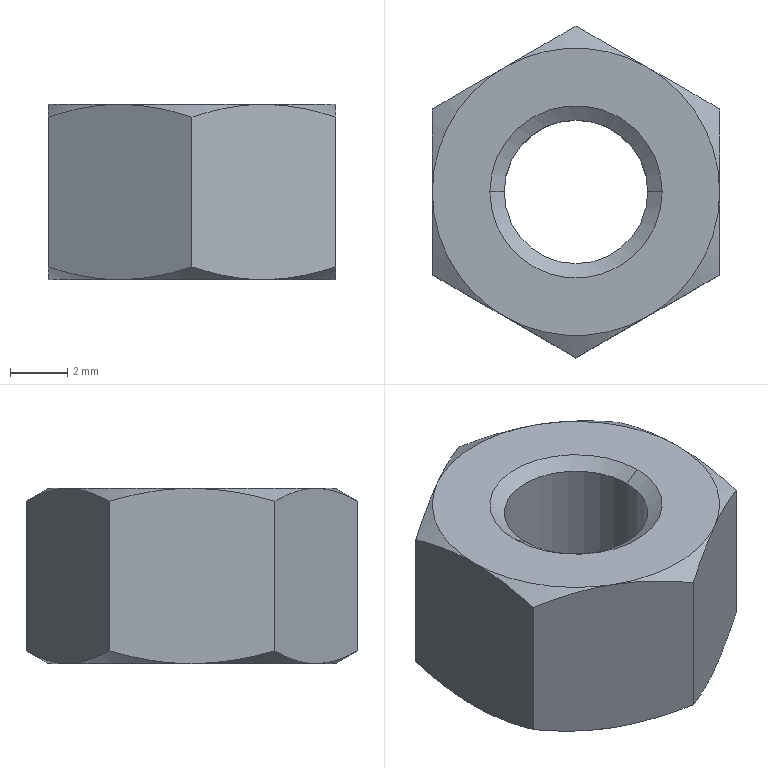Part | STEP file | hex nut gradec_iso(Hexagon Nut ISO - 4034 - M6 - N) | 1 solid | 28 faces | box 10 x 11.547 x 6.1 mm | volume 403.17 mm3 | cone 16 | plane 8 | cylinder 4 | commonest cylinder face diameters 5 x2 6 x2